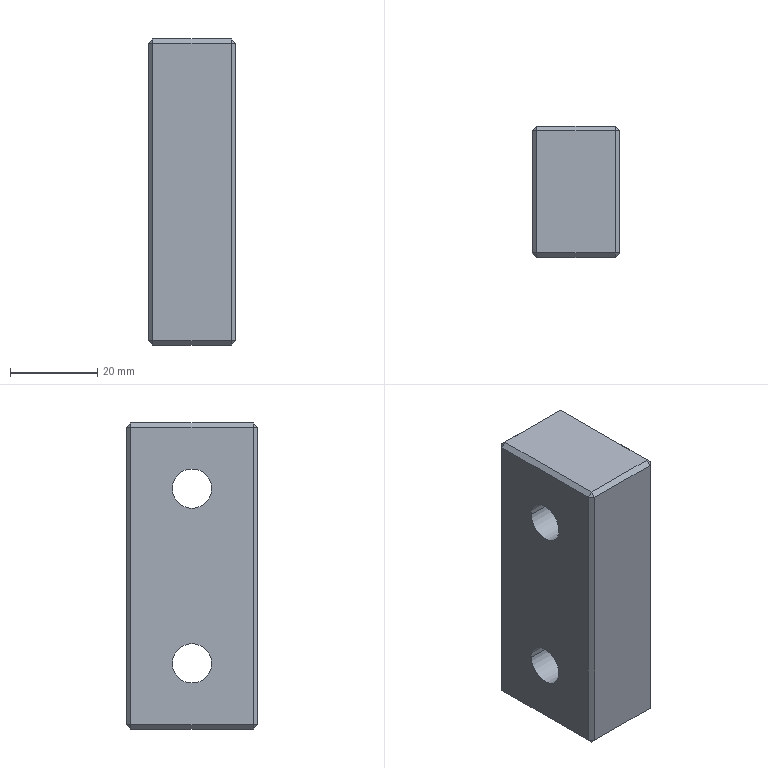Part | Creo | 1 solid | 36 faces | box 20 x 30 x 70 mm | volume 37595 mm3 | plane 28 | cylinder 8 | commonest cylinder face diameters 9 x4 14 x4
STEP:
#1=CARTESIAN_POINT('',(325.,-319.,-34.));
#2=VERTEX_POINT('',#1);
#3=CARTESIAN_POINT('',(325.,-291.,-34.));
#4=VERTEX_POINT('',#3);
#5=CARTESIAN_POINT('',(325.,-319.,-34.));
#6=DIRECTION('',(0.,1.,0.));
#7=VECTOR('',#6,28.);
#8=LINE('',#5,#7);
#9=EDGE_CURVE('',#2,#4,#8,.T.);
#10=ORIENTED_EDGE('',*,*,#9,.T.);
#11=CARTESIAN_POINT('',(325.,-291.,34.));
#12=VERTEX_POINT('',#11);
#13=CARTESIAN_POINT('',(325.,-291.,-34.));
#14=DIRECTION('',(0.,0.,1.));
#15=VECTOR('',#14,68.);
#16=LINE('',#13,#15);
#17=EDGE_CURVE('',#4,#12,#16,.T.);
#18=ORIENTED_EDGE('',*,*,#17,.T.);
#19=CARTESIAN_POINT('',(325.,-319.,34.));
#20=VERTEX_POINT('',#19);
#21=CARTESIAN_POINT('',(325.,-291.,34.));
#22=DIRECTION('',(0.,-1.,0.));
#23=VECTOR('',#22,28.);
#24=LINE('',#21,#23);
#25=EDGE_CURVE('',#12,#20,#24,.T.);
#26=ORIENTED_EDGE('',*,*,#25,.T.);
#27=CARTESIAN_POINT('',(325.,-319.,34.));
#28=DIRECTION('',(0.,0.,-1.));
#29=VECTOR('',#28,68.);
#30=LINE('',#27,#29);
#31=EDGE_CURVE('',#20,#2,#30,.T.);
#32=ORIENTED_EDGE('',*,*,#31,.T.);
#33=EDGE_LOOP('',(#10,#18,#26,#32));
#34=FACE_OUTER_BOUND('',#33,.F.);
#35=CARTESIAN_POINT('',(325.,-300.5,20.));
#36=VERTEX_POINT('',#35);
#37=CARTESIAN_POINT('',(325.,-309.5,20.));
#38=VERTEX_POINT('',#37);
#39=CARTESIAN_POINT('',(325.,-305.,20.));
#40=DIRECTION('',(1.,0.,0.));
#41=DIRECTION('',(0.,1.,0.));
#42=AXIS2_PLACEMENT_3D('',#39,#40,#41);
#43=CIRCLE('',#42,4.5);
#44=EDGE_CURVE('',#36,#38,#43,.T.);
#45=ORIENTED_EDGE('',*,*,#44,.F.);
#46=CARTESIAN_POINT('',(325.,-305.,20.));
#47=DIRECTION('',(1.,0.,0.));
#48=DIRECTION('',(0.,-1.,0.));
#49=AXIS2_PLACEMENT_3D('',#46,#47,#48);
#50=CIRCLE('',#49,4.5);
#51=EDGE_CURVE('',#38,#36,#50,.T.);
#52=ORIENTED_EDGE('',*,*,#51,.F.);
#53=EDGE_LOOP('',(#45,#52));
#54=FACE_BOUND('',#53,.F.);
#55=CARTESIAN_POINT('',(325.,-300.5,-20.));
#56=VERTEX_POINT('',#55);
#57=CARTESIAN_POINT('',(325.,-309.5,-20.));
#58=VERTEX_POINT('',#57);
#59=CARTESIAN_POINT('',(325.,-305.,-20.));
#60=DIRECTION('',(1.,0.,0.));
#61=DIRECTION('',(0.,1.,0.));
#62=AXIS2_PLACEMENT_3D('',#59,#60,#61);
#63=CIRCLE('',#62,4.5);
#64=EDGE_CURVE('',#56,#58,#63,.T.);
#65=ORIENTED_EDGE('',*,*,#64,.F.);
#66=CARTESIAN_POINT('',(325.,-305.,-20.));
#67=DIRECTION('',(1.,0.,0.));
#68=DIRECTION('',(0.,-1.,0.));
#69=AXIS2_PLACEMENT_3D('',#66,#67,#68);
#70=CIRCLE('',#69,4.5);
#71=EDGE_CURVE('',#58,#56,#70,.T.);
#72=ORIENTED_EDGE('',*,*,#71,.F.);
#73=EDGE_LOOP('',(#65,#72));
#74=FACE_BOUND('',#73,.F.);
#75=CARTESIAN_POINT('',(325.,20.,-120.5));
#76=DIRECTION('',(-1.,0.,0.));
#77=DIRECTION('',(0.,0.,-1.));
#78=AXIS2_PLACEMENT_3D('',#75,#76,#77);
#79=PLANE('',#78);
#80=ADVANCED_FACE('',(#34,#54,#74),#79,.T.);
#81=CARTESIAN_POINT('',(326.,-291.,-35.));
#82=VERTEX_POINT('',#81);
#83=CARTESIAN_POINT('',(326.,-291.,-35.));
#84=DIRECTION('',(-0.7071,0.,0.7071));
#85=VECTOR('',#84,1.414);
#86=LINE('',#83,#85);
#87=EDGE_CURVE('',#82,#4,#86,.T.);
#88=ORIENTED_EDGE('',*,*,#87,.T.);
#89=ORIENTED_EDGE('',*,*,#9,.F.);
#90=CARTESIAN_POINT('',(326.,-319.,-35.));
#91=VERTEX_POINT('',#90);
#92=CARTESIAN_POINT('',(326.,-319.,-35.));
#93=DIRECTION('',(-0.7071,0.,0.7071));
#94=VECTOR('',#93,1.414);
#95=LINE('',#92,#94);
#96=EDGE_CURVE('',#91,#2,#95,.T.);
#97=ORIENTED_EDGE('',*,*,#96,.F.);
#98=CARTESIAN_POINT('',(326.,-291.,-35.));
#99=DIRECTION('',(0.,-1.,0.));
#100=VECTOR('',#99,28.);
#101=LINE('',#98,#100);
#102=EDGE_CURVE('',#82,#91,#101,.T.);
#103=ORIENTED_EDGE('',*,*,#102,.F.);
#104=EDGE_LOOP('',(#88,#89,#97,#103));
#105=FACE_OUTER_BOUND('',#104,.F.);
#106=CARTESIAN_POINT('',(326.,20.,-35.));
#107=DIRECTION('',(-0.7071,0.,-0.7071));
#108=DIRECTION('',(0.7071,0.,-0.7071));
#109=AXIS2_PLACEMENT_3D('',#106,#107,#108);
#110=PLANE('',#109);
#111=ADVANCED_FACE('',(#105),#110,.T.);
#112=CARTESIAN_POINT('',(326.,-290.,-34.));
#113=VERTEX_POINT('',#112);
#114=CARTESIAN_POINT('',(325.,-291.,-34.));
#115=DIRECTION('',(0.7071,0.7071,0.));
#116=VECTOR('',#115,1.414);
#117=LINE('',#114,#116);
#118=EDGE_CURVE('',#4,#113,#117,.T.);
#119=ORIENTED_EDGE('',*,*,#118,.F.);
#120=ORIENTED_EDGE('',*,*,#87,.F.);
#121=CARTESIAN_POINT('',(326.,-290.,-34.));
#122=DIRECTION('',(0.,-0.7071,-0.7071));
#123=VECTOR('',#122,1.414);
#124=LINE('',#121,#123);
#125=EDGE_CURVE('',#113,#82,#124,.T.);
#126=ORIENTED_EDGE('',*,*,#125,.F.);
#127=EDGE_LOOP('',(#119,#120,#126));
#128=FACE_OUTER_BOUND('',#127,.F.);
#129=CARTESIAN_POINT('',(326.,-291.,-35.));
#130=DIRECTION('',(-0.5774,0.5774,-0.5774));
#131=DIRECTION('',(0.7071,0.,-0.7071));
#132=AXIS2_PLACEMENT_3D('',#129,#130,#131);
#133=PLANE('',#132);
#134=ADVANCED_FACE('',(#128),#133,.T.);
#135=ORIENTED_EDGE('',*,*,#118,.T.);
#136=CARTESIAN_POINT('',(326.,-290.,34.));
#137=VERTEX_POINT('',#136);
#138=CARTESIAN_POINT('',(326.,-290.,34.));
#139=DIRECTION('',(0.,0.,-1.));
#140=VECTOR('',#139,68.);
#141=LINE('',#138,#140);
#142=EDGE_CURVE('',#137,#113,#141,.T.);
#143=ORIENTED_EDGE('',*,*,#142,.F.);
#144=CARTESIAN_POINT('',(326.,-290.,34.));
#145=DIRECTION('',(-0.7071,-0.7071,0.));
#146=VECTOR('',#145,1.414);
#147=LINE('',#144,#146);
#148=EDGE_CURVE('',#137,#12,#147,.T.);
#149=ORIENTED_EDGE('',*,*,#148,.T.);
#150=ORIENTED_EDGE('',*,*,#17,.F.);
#151=EDGE_LOOP('',(#135,#143,#149,#150));
#152=FACE_OUTER_BOUND('',#151,.F.);
#153=CARTESIAN_POINT('',(326.,-290.,20.));
#154=DIRECTION('',(-0.7071,0.7071,0.));
#155=DIRECTION('',(-0.7071,-0.7071,0.));
#156=AXIS2_PLACEMENT_3D('',#153,#154,#155);
#157=PLANE('',#156);
#158=ADVANCED_FACE('',(#152),#157,.T.);
#159=CARTESIAN_POINT('',(344.,-290.,-34.));
#160=VERTEX_POINT('',#159);
#161=CARTESIAN_POINT('',(344.,-290.,34.));
#162=VERTEX_POINT('',#161);
#163=CARTESIAN_POINT('',(344.,-290.,-34.));
#164=DIRECTION('',(0.,0.,1.));
#165=VECTOR('',#164,68.);
#166=LINE('',#163,#165);
#167=EDGE_CURVE('',#160,#162,#166,.T.);
#168=ORIENTED_EDGE('',*,*,#167,.T.);
#169=CARTESIAN_POINT('',(344.,-290.,34.));
#170=DIRECTION('',(-1.,0.,0.));
#171=VECTOR('',#170,18.);
#172=LINE('',#169,#171);
#173=EDGE_CURVE('',#162,#137,#172,.T.);
#174=ORIENTED_EDGE('',*,*,#173,.T.);
#175=ORIENTED_EDGE('',*,*,#142,.T.);
#176=CARTESIAN_POINT('',(326.,-290.,-34.));
#177=DIRECTION('',(1.,0.,0.));
#178=VECTOR('',#177,18.);
#179=LINE('',#176,#178);
#180=EDGE_CURVE('',#113,#160,#179,.T.);
#181=ORIENTED_EDGE('',*,*,#180,.T.);
#182=EDGE_LOOP('',(#168,#174,#175,#181));
#183=FACE_OUTER_BOUND('',#182,.F.);
#184=CARTESIAN_POINT('',(335.,-290.,20.));
#185=DIRECTION('',(0.,-1.,0.));
#186=DIRECTION('',(0.,0.,1.));
#187=AXIS2_PLACEMENT_3D('',#184,#185,#186);
#188=PLANE('',#187);
#189=ADVANCED_FACE('',(#183),#188,.F.);
#190=CARTESIAN_POINT('',(345.,-291.,-34.));
#191=VERTEX_POINT('',#190);
#192=CARTESIAN_POINT('',(344.,-290.,-34.));
#193=DIRECTION('',(0.7071,-0.7071,0.));
#194=VECTOR('',#193,1.414);
#195=LINE('',#192,#194);
#196=EDGE_CURVE('',#160,#191,#195,.T.);
#197=ORIENTED_EDGE('',*,*,#196,.T.);
#198=CARTESIAN_POINT('',(345.,-291.,34.));
#199=VERTEX_POINT('',#198);
#200=CARTESIAN_POINT('',(345.,-291.,34.));
#201=DIRECTION('',(0.,0.,-1.));
#202=VECTOR('',#201,68.);
#203=LINE('',#200,#202);
#204=EDGE_CURVE('',#199,#191,#203,.T.);
#205=ORIENTED_EDGE('',*,*,#204,.F.);
#206=CARTESIAN_POINT('',(345.,-291.,34.));
#207=DIRECTION('',(-0.7071,0.7071,0.));
#208=VECTOR('',#207,1.414);
#209=LINE('',#206,#208);
#210=EDGE_CURVE('',#199,#162,#209,.T.);
#211=ORIENTED_EDGE('',*,*,#210,.T.);
#212=ORIENTED_EDGE('',*,*,#167,.F.);
#213=EDGE_LOOP('',(#197,#205,#211,#212));
#214=FACE_OUTER_BOUND('',#213,.F.);
#215=CARTESIAN_POINT('',(344.,-290.,20.));
#216=DIRECTION('',(0.7071,0.7071,0.));
#217=DIRECTION('',(-0.7071,0.7071,0.));
#218=AXIS2_PLACEMENT_3D('',#215,#216,#217);
#219=PLANE('',#218);
#220=ADVANCED_FACE('',(#214),#219,.T.);
#221=CARTESIAN_POINT('',(344.,-291.,-35.));
#222=VERTEX_POINT('',#221);
#223=CARTESIAN_POINT('',(345.,-291.,-34.));
#224=DIRECTION('',(-0.7071,0.,-0.7071));
#225=VECTOR('',#224,1.414);
#226=LINE('',#223,#225);
#227=EDGE_CURVE('',#191,#222,#226,.T.);
#228=ORIENTED_EDGE('',*,*,#227,.F.);
#229=ORIENTED_EDGE('',*,*,#196,.F.);
#230=CARTESIAN_POINT('',(344.,-291.,-35.));
#231=DIRECTION('',(0.,0.7071,0.7071));
#232=VECTOR('',#231,1.414);
#233=LINE('',#230,#232);
#234=EDGE_CURVE('',#222,#160,#233,.T.);
#235=ORIENTED_EDGE('',*,*,#234,.F.);
#236=EDGE_LOOP('',(#228,#229,#235));
#237=FACE_OUTER_BOUND('',#236,.F.);
#238=CARTESIAN_POINT('',(344.,-291.,-35.));
#239=DIRECTION('',(0.5774,0.5774,-0.5774));
#240=DIRECTION('',(0.7071,0.,0.7071));
#241=AXIS2_PLACEMENT_3D('',#238,#239,#240);
#242=PLANE('',#241);
#243=ADVANCED_FACE('',(#237),#242,.T.);
#244=ORIENTED_EDGE('',*,*,#227,.T.);
#245=CARTESIAN_POINT('',(344.,-319.,-35.));
#246=VERTEX_POINT('',#245);
#247=CARTESIAN_POINT('',(344.,-319.,-35.));
#248=DIRECTION('',(0.,1.,0.));
#249=VECTOR('',#248,28.);
#250=LINE('',#247,#249);
#251=EDGE_CURVE('',#246,#222,#250,.T.);
#252=ORIENTED_EDGE('',*,*,#251,.F.);
#253=CARTESIAN_POINT('',(345.,-319.,-34.));
#254=VERTEX_POINT('',#253);
#255=CARTESIAN_POINT('',(345.,-319.,-34.));
#256=DIRECTION('',(-0.7071,0.,-0.7071));
#257=VECTOR('',#256,1.414);
#258=LINE('',#255,#257);
#259=EDGE_CURVE('',#254,#246,#258,.T.);
#260=ORIENTED_EDGE('',*,*,#259,.F.);
#261=CARTESIAN_POINT('',(345.,-291.,-34.));
#262=DIRECTION('',(0.,-1.,0.));
#263=VECTOR('',#262,28.);
#264=LINE('',#261,#263);
#265=EDGE_CURVE('',#191,#254,#264,.T.);
#266=ORIENTED_EDGE('',*,*,#265,.F.);
#267=EDGE_LOOP('',(#244,#252,#260,#266));
#268=FACE_OUTER_BOUND('',#267,.F.);
#269=CARTESIAN_POINT('',(344.,20.,-35.));
#270=DIRECTION('',(0.7071,0.,-0.7071));
#271=DIRECTION('',(0.7071,0.,0.7071));
#272=AXIS2_PLACEMENT_3D('',#269,#270,#271);
#273=PLANE('',#272);
#274=ADVANCED_FACE('',(#268),#273,.T.);
#275=ORIENTED_EDGE('',*,*,#251,.T.);
#276=CARTESIAN_POINT('',(344.,-291.,-35.));
#277=DIRECTION('',(-1.,0.,0.));
#278=VECTOR('',#277,18.);
#279=LINE('',#276,#278);
#280=EDGE_CURVE('',#222,#82,#279,.T.);
#281=ORIENTED_EDGE('',*,*,#280,.T.);
#282=ORIENTED_EDGE('',*,*,#102,.T.);
#283=CARTESIAN_POINT('',(326.,-319.,-35.));
#284=DIRECTION('',(1.,0.,0.));
#285=VECTOR('',#284,18.);
#286=LINE('',#283,#285);
#287=EDGE_CURVE('',#91,#246,#286,.T.);
#288=ORIENTED_EDGE('',*,*,#287,.T.);
#289=EDGE_LOOP('',(#275,#281,#282,#288));
#290=FACE_OUTER_BOUND('',#289,.F.);
#291=CARTESIAN_POINT('',(0.,20.,-35.));
#292=DIRECTION('',(0.,0.,1.));
#293=DIRECTION('',(-1.,0.,0.));
#294=AXIS2_PLACEMENT_3D('',#291,#292,#293);
#295=PLANE('',#294);
#296=ADVANCED_FACE('',(#290),#295,.F.);
#297=ORIENTED_EDGE('',*,*,#234,.T.);
#298=ORIENTED_EDGE('',*,*,#180,.F.);
#299=ORIENTED_EDGE('',*,*,#125,.T.);
#300=ORIENTED_EDGE('',*,*,#280,.F.);
#301=EDGE_LOOP('',(#297,#298,#299,#300));
#302=FACE_OUTER_BOUND('',#301,.F.);
#303=CARTESIAN_POINT('',(335.,-290.,-34.));
#304=DIRECTION('',(0.,-0.7071,0.7071));
#305=DIRECTION('',(0.,0.7071,0.7071));
#306=AXIS2_PLACEMENT_3D('',#303,#304,#305);
#307=PLANE('',#306);
#308=ADVANCED_FACE('',(#302),#307,.F.);
#309=CARTESIAN_POINT('',(326.,-320.,-34.));
#310=VERTEX_POINT('',#309);
#311=CARTESIAN_POINT('',(326.,-319.,-35.));
#312=DIRECTION('',(0.,-0.7071,0.7071));
#313=VECTOR('',#312,1.414);
#314=LINE('',#311,#313);
#315=EDGE_CURVE('',#91,#310,#314,.T.);
#316=ORIENTED_EDGE('',*,*,#315,.T.);
#317=CARTESIAN_POINT('',(344.,-320.,-34.));
#318=VERTEX_POINT('',#317);
#319=CARTESIAN_POINT('',(344.,-320.,-34.));
#320=DIRECTION('',(-1.,0.,0.));
#321=VECTOR('',#320,18.);
#322=LINE('',#319,#321);
#323=EDGE_CURVE('',#318,#310,#322,.T.);
#324=ORIENTED_EDGE('',*,*,#323,.F.);
#325=CARTESIAN_POINT('',(344.,-320.,-34.));
#326=DIRECTION('',(0.,0.7071,-0.7071));
#327=VECTOR('',#326,1.414);
#328=LINE('',#325,#327);
#329=EDGE_CURVE('',#318,#246,#328,.T.);
#330=ORIENTED_EDGE('',*,*,#329,.T.);
#331=ORIENTED_EDGE('',*,*,#287,.F.);
#332=EDGE_LOOP('',(#316,#324,#330,#331));
#333=FACE_OUTER_BOUND('',#332,.F.);
#334=CARTESIAN_POINT('',(0.,-319.,-35.));
#335=DIRECTION('',(0.,-0.7071,-0.7071));
#336=DIRECTION('',(0.,-0.7071,0.7071));
#337=AXIS2_PLACEMENT_3D('',#334,#335,#336);
#338=PLANE('',#337);
#339=ADVANCED_FACE('',(#333),#338,.T.);
#340=ORIENTED_EDGE('',*,*,#96,.T.);
#341=CARTESIAN_POINT('',(326.,-320.,-34.));
#342=DIRECTION('',(-0.7071,0.7071,0.));
#343=VECTOR('',#342,1.414);
#344=LINE('',#341,#343);
#345=EDGE_CURVE('',#310,#2,#344,.T.);
#346=ORIENTED_EDGE('',*,*,#345,.F.);
#347=ORIENTED_EDGE('',*,*,#315,.F.);
#348=EDGE_LOOP('',(#340,#346,#347));
#349=FACE_OUTER_BOUND('',#348,.F.);
#350=CARTESIAN_POINT('',(326.,-320.,-34.));
#351=DIRECTION('',(-0.5774,-0.5774,-0.5774));
#352=DIRECTION('',(0.7071,0.,-0.7071));
#353=AXIS2_PLACEMENT_3D('',#350,#351,#352);
#354=PLANE('',#353);
#355=ADVANCED_FACE('',(#349),#354,.T.);
#356=ORIENTED_EDGE('',*,*,#345,.T.);
#357=ORIENTED_EDGE('',*,*,#31,.F.);
#358=CARTESIAN_POINT('',(326.,-320.,34.));
#359=VERTEX_POINT('',#358);
#360=CARTESIAN_POINT('',(325.,-319.,34.));
#361=DIRECTION('',(0.7071,-0.7071,0.));
#362=VECTOR('',#361,1.414);
#363=LINE('',#360,#362);
#364=EDGE_CURVE('',#20,#359,#363,.T.);
#365=ORIENTED_EDGE('',*,*,#364,.T.);
#366=CARTESIAN_POINT('',(326.,-320.,-34.));
#367=DIRECTION('',(0.,0.,1.));
#368=VECTOR('',#367,68.);
#369=LINE('',#366,#368);
#370=EDGE_CURVE('',#310,#359,#369,.T.);
#371=ORIENTED_EDGE('',*,*,#370,.F.);
#372=EDGE_LOOP('',(#356,#357,#365,#371));
#373=FACE_OUTER_BOUND('',#372,.F.);
#374=CARTESIAN_POINT('',(325.,-319.,-120.5));
#375=DIRECTION('',(0.7071,0.7071,0.));
#376=DIRECTION('',(-0.7071,0.7071,0.));
#377=AXIS2_PLACEMENT_3D('',#374,#375,#376);
#378=PLANE('',#377);
#379=ADVANCED_FACE('',(#373),#378,.F.);
#380=CARTESIAN_POINT('',(326.,-319.,35.));
#381=VERTEX_POINT('',#380);
#382=CARTESIAN_POINT('',(325.,-319.,34.));
#383=DIRECTION('',(0.7071,0.,0.7071));
#384=VECTOR('',#383,1.414);
#385=LINE('',#382,#384);
#386=EDGE_CURVE('',#20,#381,#385,.T.);
#387=ORIENTED_EDGE('',*,*,#386,.T.);
#388=CARTESIAN_POINT('',(326.,-320.,34.));
#389=DIRECTION('',(0.,0.7071,0.7071));
#390=VECTOR('',#389,1.414);
#391=LINE('',#388,#390);
#392=EDGE_CURVE('',#359,#381,#391,.T.);
#393=ORIENTED_EDGE('',*,*,#392,.F.);
#394=ORIENTED_EDGE('',*,*,#364,.F.);
#395=EDGE_LOOP('',(#387,#393,#394));
#396=FACE_OUTER_BOUND('',#395,.F.);
#397=CARTESIAN_POINT('',(326.,-320.,34.));
#398=DIRECTION('',(-0.5774,-0.5774,0.5774));
#399=DIRECTION('',(-0.7071,0.,-0.7071));
#400=AXIS2_PLACEMENT_3D('',#397,#398,#399);
#401=PLANE('',#400);
#402=ADVANCED_FACE('',(#396),#401,.T.);
#403=CARTESIAN_POINT('',(326.,-291.,35.));
#404=VERTEX_POINT('',#403);
#405=CARTESIAN_POINT('',(325.,-291.,34.));
#406=DIRECTION('',(0.7071,0.,0.7071));
#407=VECTOR('',#406,1.414);
#408=LINE('',#405,#407);
#409=EDGE_CURVE('',#12,#404,#408,.T.);
#410=ORIENTED_EDGE('',*,*,#409,.T.);
#411=CARTESIAN_POINT('',(326.,-319.,35.));
#412=DIRECTION('',(0.,1.,0.));
#413=VECTOR('',#412,28.);
#414=LINE('',#411,#413);
#415=EDGE_CURVE('',#381,#404,#414,.T.);
#416=ORIENTED_EDGE('',*,*,#415,.F.);
#417=ORIENTED_EDGE('',*,*,#386,.F.);
#418=ORIENTED_EDGE('',*,*,#25,.F.);
#419=EDGE_LOOP('',(#410,#416,#417,#418));
#420=FACE_OUTER_BOUND('',#419,.F.);
#421=CARTESIAN_POINT('',(325.,20.,34.));
#422=DIRECTION('',(0.7071,0.,-0.7071));
#423=DIRECTION('',(0.7071,0.,0.7071));
#424=AXIS2_PLACEMENT_3D('',#421,#422,#423);
#425=PLANE('',#424);
#426=ADVANCED_FACE('',(#420),#425,.F.);
#427=CARTESIAN_POINT('',(326.,-291.,35.));
#428=DIRECTION('',(0.,0.7071,-0.7071));
#429=VECTOR('',#428,1.414);
#430=LINE('',#427,#429);
#431=EDGE_CURVE('',#404,#137,#430,.T.);
#432=ORIENTED_EDGE('',*,*,#431,.F.);
#433=ORIENTED_EDGE('',*,*,#409,.F.);
#434=ORIENTED_EDGE('',*,*,#148,.F.);
#435=EDGE_LOOP('',(#432,#433,#434));
#436=FACE_OUTER_BOUND('',#435,.F.);
#437=CARTESIAN_POINT('',(326.,-290.,34.));
#438=DIRECTION('',(-0.5774,0.5774,0.5774));
#439=DIRECTION('',(-0.7071,0.,-0.7071));
#440=AXIS2_PLACEMENT_3D('',#437,#438,#439);
#441=PLANE('',#440);
#442=ADVANCED_FACE('',(#436),#441,.T.);
#443=CARTESIAN_POINT('',(344.,-291.,35.));
#444=VERTEX_POINT('',#443);
#445=CARTESIAN_POINT('',(344.,-290.,34.));
#446=DIRECTION('',(0.,-0.7071,0.7071));
#447=VECTOR('',#446,1.414);
#448=LINE('',#445,#447);
#449=EDGE_CURVE('',#162,#444,#448,.T.);
#450=ORIENTED_EDGE('',*,*,#449,.T.);
#451=CARTESIAN_POINT('',(326.,-291.,35.));
#452=DIRECTION('',(1.,0.,0.));
#453=VECTOR('',#452,18.);
#454=LINE('',#451,#453);
#455=EDGE_CURVE('',#404,#444,#454,.T.);
#456=ORIENTED_EDGE('',*,*,#455,.F.);
#457=ORIENTED_EDGE('',*,*,#431,.T.);
#458=ORIENTED_EDGE('',*,*,#173,.F.);
#459=EDGE_LOOP('',(#450,#456,#457,#458));
#460=FACE_OUTER_BOUND('',#459,.F.);
#461=CARTESIAN_POINT('',(0.,-291.,35.));
#462=DIRECTION('',(0.,0.7071,0.7071));
#463=DIRECTION('',(0.,0.7071,-0.7071));
#464=AXIS2_PLACEMENT_3D('',#461,#462,#463);
#465=PLANE('',#464);
#466=ADVANCED_FACE('',(#460),#465,.T.);
#467=ORIENTED_EDGE('',*,*,#210,.F.);
#468=CARTESIAN_POINT('',(344.,-291.,35.));
#469=DIRECTION('',(0.7071,0.,-0.7071));
#470=VECTOR('',#469,1.414);
#471=LINE('',#468,#470);
#472=EDGE_CURVE('',#444,#199,#471,.T.);
#473=ORIENTED_EDGE('',*,*,#472,.F.);
#474=ORIENTED_EDGE('',*,*,#449,.F.);
#475=EDGE_LOOP('',(#467,#473,#474));
#476=FACE_OUTER_BOUND('',#475,.F.);
#477=CARTESIAN_POINT('',(345.,-291.,34.));
#478=DIRECTION('',(0.5774,0.5774,0.5774));
#479=DIRECTION('',(-0.7071,0.,0.7071));
#480=AXIS2_PLACEMENT_3D('',#477,#478,#479);
#481=PLANE('',#480);
#482=ADVANCED_FACE('',(#476),#481,.T.);
#483=ORIENTED_EDGE('',*,*,#472,.T.);
#484=CARTESIAN_POINT('',(345.,-319.,34.));
#485=VERTEX_POINT('',#484);
#486=CARTESIAN_POINT('',(345.,-319.,34.));
#487=DIRECTION('',(0.,1.,0.));
#488=VECTOR('',#487,28.);
#489=LINE('',#486,#488);
#490=EDGE_CURVE('',#485,#199,#489,.T.);
#491=ORIENTED_EDGE('',*,*,#490,.F.);
#492=CARTESIAN_POINT('',(344.,-319.,35.));
#493=VERTEX_POINT('',#492);
#494=CARTESIAN_POINT('',(344.,-319.,35.));
#495=DIRECTION('',(0.7071,0.,-0.7071));
#496=VECTOR('',#495,1.414);
#497=LINE('',#494,#496);
#498=EDGE_CURVE('',#493,#485,#497,.T.);
#499=ORIENTED_EDGE('',*,*,#498,.F.);
#500=CARTESIAN_POINT('',(344.,-291.,35.));
#501=DIRECTION('',(0.,-1.,0.));
#502=VECTOR('',#501,28.);
#503=LINE('',#500,#502);
#504=EDGE_CURVE('',#444,#493,#503,.T.);
#505=ORIENTED_EDGE('',*,*,#504,.F.);
#506=EDGE_LOOP('',(#483,#491,#499,#505));
#507=FACE_OUTER_BOUND('',#506,.F.);
#508=CARTESIAN_POINT('',(345.,20.,34.));
#509=DIRECTION('',(-0.7071,0.,-0.7071));
#510=DIRECTION('',(0.7071,0.,-0.7071));
#511=AXIS2_PLACEMENT_3D('',#508,#509,#510);
#512=PLANE('',#511);
#513=ADVANCED_FACE('',(#507),#512,.F.);
#514=CARTESIAN_POINT('',(345.,-319.,-34.));
#515=DIRECTION('',(0.,0.,1.));
#516=VECTOR('',#515,68.);
#517=LINE('',#514,#516);
#518=EDGE_CURVE('',#254,#485,#517,.T.);
#519=ORIENTED_EDGE('',*,*,#518,.T.);
#520=ORIENTED_EDGE('',*,*,#490,.T.);
#521=ORIENTED_EDGE('',*,*,#204,.T.);
#522=ORIENTED_EDGE('',*,*,#265,.T.);
#523=EDGE_LOOP('',(#519,#520,#521,#522));
#524=FACE_OUTER_BOUND('',#523,.F.);
#525=CARTESIAN_POINT('',(345.,-298.,-20.));
#526=VERTEX_POINT('',#525);
#527=CARTESIAN_POINT('',(345.,-312.,-20.));
#528=VERTEX_POINT('',#527);
#529=CARTESIAN_POINT('',(345.,-305.,-20.));
#530=DIRECTION('',(-1.,0.,0.));
#531=DIRECTION('',(0.,1.,0.));
#532=AXIS2_PLACEMENT_3D('',#529,#530,#531);
#533=CIRCLE('',#532,7.);
#534=EDGE_CURVE('',#526,#528,#533,.T.);
#535=ORIENTED_EDGE('',*,*,#534,.F.);
#536=CARTESIAN_POINT('',(345.,-305.,-20.));
#537=DIRECTION('',(-1.,0.,0.));
#538=DIRECTION('',(0.,-1.,0.));
#539=AXIS2_PLACEMENT_3D('',#536,#537,#538);
#540=CIRCLE('',#539,7.);
#541=EDGE_CURVE('',#528,#526,#540,.T.);
#542=ORIENTED_EDGE('',*,*,#541,.F.);
#543=EDGE_LOOP('',(#535,#542));
#544=FACE_BOUND('',#543,.F.);
#545=CARTESIAN_POINT('',(345.,-298.,20.));
#546=VERTEX_POINT('',#545);
#547=CARTESIAN_POINT('',(345.,-312.,20.));
#548=VERTEX_POINT('',#547);
#549=CARTESIAN_POINT('',(345.,-305.,20.));
#550=DIRECTION('',(-1.,0.,0.));
#551=DIRECTION('',(0.,1.,0.));
#552=AXIS2_PLACEMENT_3D('',#549,#550,#551);
#553=CIRCLE('',#552,7.);
#554=EDGE_CURVE('',#546,#548,#553,.T.);
#555=ORIENTED_EDGE('',*,*,#554,.F.);
#556=CARTESIAN_POINT('',(345.,-305.,20.));
#557=DIRECTION('',(-1.,0.,0.));
#558=DIRECTION('',(0.,-1.,0.));
#559=AXIS2_PLACEMENT_3D('',#556,#557,#558);
#560=CIRCLE('',#559,7.);
#561=EDGE_CURVE('',#548,#546,#560,.T.);
#562=ORIENTED_EDGE('',*,*,#561,.F.);
#563=EDGE_LOOP('',(#555,#562));
#564=FACE_BOUND('',#563,.F.);
#565=CARTESIAN_POINT('',(345.,20.,-120.5));
#566=DIRECTION('',(1.,0.,0.));
#567=DIRECTION('',(0.,0.,1.));
#568=AXIS2_PLACEMENT_3D('',#565,#566,#567);
#569=PLANE('',#568);
#570=ADVANCED_FACE('',(#524,#544,#564),#569,.T.);
#571=CARTESIAN_POINT('',(345.,-319.,-34.));
#572=DIRECTION('',(-0.7071,-0.7071,0.));
#573=VECTOR('',#572,1.414);
#574=LINE('',#571,#573);
#575=EDGE_CURVE('',#254,#318,#574,.T.);
#576=ORIENTED_EDGE('',*,*,#575,.T.);
#577=CARTESIAN_POINT('',(344.,-320.,34.));
#578=VERTEX_POINT('',#577);
#579=CARTESIAN_POINT('',(344.,-320.,34.));
#580=DIRECTION('',(0.,0.,-1.));
#581=VECTOR('',#580,68.);
#582=LINE('',#579,#581);
#583=EDGE_CURVE('',#578,#318,#582,.T.);
#584=ORIENTED_EDGE('',*,*,#583,.F.);
#585=CARTESIAN_POINT('',(344.,-320.,34.));
#586=DIRECTION('',(0.7071,0.7071,0.));
#587=VECTOR('',#586,1.414);
#588=LINE('',#585,#587);
#589=EDGE_CURVE('',#578,#485,#588,.T.);
#590=ORIENTED_EDGE('',*,*,#589,.T.);
#591=ORIENTED_EDGE('',*,*,#518,.F.);
#592=EDGE_LOOP('',(#576,#584,#590,#591));
#593=FACE_OUTER_BOUND('',#592,.F.);
#594=CARTESIAN_POINT('',(345.,-319.,-120.5));
#595=DIRECTION('',(-0.7071,0.7071,0.));
#596=DIRECTION('',(-0.7071,-0.7071,0.));
#597=AXIS2_PLACEMENT_3D('',#594,#595,#596);
#598=PLANE('',#597);
#599=ADVANCED_FACE('',(#593),#598,.F.);
#600=ORIENTED_EDGE('',*,*,#329,.F.);
#601=ORIENTED_EDGE('',*,*,#575,.F.);
#602=ORIENTED_EDGE('',*,*,#259,.T.);
#603=EDGE_LOOP('',(#600,#601,#602));
#604=FACE_OUTER_BOUND('',#603,.F.);
#605=CARTESIAN_POINT('',(344.,-320.,-34.));
#606=DIRECTION('',(0.5774,-0.5774,-0.5774));
#607=DIRECTION('',(0.7071,0.,0.7071));
#608=AXIS2_PLACEMENT_3D('',#605,#606,#607);
#609=PLANE('',#608);
#610=ADVANCED_FACE('',(#604),#609,.T.);
#611=ORIENTED_EDGE('',*,*,#583,.T.);
#612=ORIENTED_EDGE('',*,*,#323,.T.);
#613=ORIENTED_EDGE('',*,*,#370,.T.);
#614=CARTESIAN_POINT('',(326.,-320.,34.));
#615=DIRECTION('',(1.,0.,0.));
#616=VECTOR('',#615,18.);
#617=LINE('',#614,#616);
#618=EDGE_CURVE('',#359,#578,#617,.T.);
#619=ORIENTED_EDGE('',*,*,#618,.T.);
#620=EDGE_LOOP('',(#611,#612,#613,#619));
#621=FACE_OUTER_BOUND('',#620,.F.);
#622=CARTESIAN_POINT('',(335.,-320.,20.));
#623=DIRECTION('',(0.,-1.,0.));
#624=DIRECTION('',(0.,0.,1.));
#625=AXIS2_PLACEMENT_3D('',#622,#623,#624);
#626=PLANE('',#625);
#627=ADVANCED_FACE('',(#621),#626,.T.);
#628=CARTESIAN_POINT('',(344.,-319.,35.));
#629=DIRECTION('',(0.,-0.7071,-0.7071));
#630=VECTOR('',#629,1.414);
#631=LINE('',#628,#630);
#632=EDGE_CURVE('',#493,#578,#631,.T.);
#633=ORIENTED_EDGE('',*,*,#632,.T.);
#634=ORIENTED_EDGE('',*,*,#618,.F.);
#635=ORIENTED_EDGE('',*,*,#392,.T.);
#636=CARTESIAN_POINT('',(344.,-319.,35.));
#637=DIRECTION('',(-1.,0.,0.));
#638=VECTOR('',#637,18.);
#639=LINE('',#636,#638);
#640=EDGE_CURVE('',#493,#381,#639,.T.);
#641=ORIENTED_EDGE('',*,*,#640,.F.);
#642=EDGE_LOOP('',(#633,#634,#635,#641));
#643=FACE_OUTER_BOUND('',#642,.F.);
#644=CARTESIAN_POINT('',(335.,-320.,34.));
#645=DIRECTION('',(0.,0.7071,-0.7071));
#646=DIRECTION('',(0.,-0.7071,-0.7071));
#647=AXIS2_PLACEMENT_3D('',#644,#645,#646);
#648=PLANE('',#647);
#649=ADVANCED_FACE('',(#643),#648,.F.);
#650=ORIENTED_EDGE('',*,*,#589,.F.);
#651=ORIENTED_EDGE('',*,*,#632,.F.);
#652=ORIENTED_EDGE('',*,*,#498,.T.);
#653=EDGE_LOOP('',(#650,#651,#652));
#654=FACE_OUTER_BOUND('',#653,.F.);
#655=CARTESIAN_POINT('',(344.,-319.,35.));
#656=DIRECTION('',(0.5774,-0.5774,0.5774));
#657=DIRECTION('',(-0.7071,0.,0.7071));
#658=AXIS2_PLACEMENT_3D('',#655,#656,#657);
#659=PLANE('',#658);
#660=ADVANCED_FACE('',(#654),#659,.T.);
#661=ORIENTED_EDGE('',*,*,#415,.T.);
#662=ORIENTED_EDGE('',*,*,#455,.T.);
#663=ORIENTED_EDGE('',*,*,#504,.T.);
#664=ORIENTED_EDGE('',*,*,#640,.T.);
#665=EDGE_LOOP('',(#661,#662,#663,#664));
#666=FACE_OUTER_BOUND('',#665,.F.);
#667=CARTESIAN_POINT('',(0.,20.,35.));
#668=DIRECTION('',(0.,0.,1.));
#669=DIRECTION('',(-1.,0.,0.));
#670=AXIS2_PLACEMENT_3D('',#667,#668,#669);
#671=PLANE('',#670);
#672=ADVANCED_FACE('',(#666),#671,.T.);
#673=ORIENTED_EDGE('',*,*,#534,.T.);
#674=CARTESIAN_POINT('',(336.,-312.,-20.));
#675=VERTEX_POINT('',#674);
#676=CARTESIAN_POINT('',(336.,-312.,-20.));
#677=DIRECTION('',(1.,0.,0.));
#678=VECTOR('',#677,9.);
#679=LINE('',#676,#678);
#680=EDGE_CURVE('',#675,#528,#679,.T.);
#681=ORIENTED_EDGE('',*,*,#680,.F.);
#682=CARTESIAN_POINT('',(336.,-298.,-20.));
#683=VERTEX_POINT('',#682);
#684=CARTESIAN_POINT('',(336.,-305.,-20.));
#685=DIRECTION('',(1.,0.,0.));
#686=DIRECTION('',(0.,-1.,0.));
#687=AXIS2_PLACEMENT_3D('',#684,#685,#686);
#688=CIRCLE('',#687,7.);
#689=EDGE_CURVE('',#675,#683,#688,.T.);
#690=ORIENTED_EDGE('',*,*,#689,.T.);
#691=CARTESIAN_POINT('',(336.,-298.,-20.));
#692=DIRECTION('',(1.,0.,0.));
#693=VECTOR('',#692,9.);
#694=LINE('',#691,#693);
#695=EDGE_CURVE('',#683,#526,#694,.T.);
#696=ORIENTED_EDGE('',*,*,#695,.T.);
#697=EDGE_LOOP('',(#673,#681,#690,#696));
#698=FACE_OUTER_BOUND('',#697,.F.);
#699=CARTESIAN_POINT('',(336.,-305.,-20.));
#700=DIRECTION('',(1.,0.,0.));
#701=DIRECTION('',(0.,1.,0.));
#702=AXIS2_PLACEMENT_3D('',#699,#700,#701);
#703=CYLINDRICAL_SURFACE('',#702,7.);
#704=ADVANCED_FACE('',(#698),#703,.F.);
#705=ORIENTED_EDGE('',*,*,#541,.T.);
#706=ORIENTED_EDGE('',*,*,#695,.F.);
#707=CARTESIAN_POINT('',(336.,-305.,-20.));
#708=DIRECTION('',(1.,0.,0.));
#709=DIRECTION('',(0.,1.,0.));
#710=AXIS2_PLACEMENT_3D('',#707,#708,#709);
#711=CIRCLE('',#710,7.);
#712=EDGE_CURVE('',#683,#675,#711,.T.);
#713=ORIENTED_EDGE('',*,*,#712,.T.);
#714=ORIENTED_EDGE('',*,*,#680,.T.);
#715=EDGE_LOOP('',(#705,#706,#713,#714));
#716=FACE_OUTER_BOUND('',#715,.F.);
#717=CARTESIAN_POINT('',(336.,-305.,-20.));
#718=DIRECTION('',(1.,0.,0.));
#719=DIRECTION('',(0.,1.,0.));
#720=AXIS2_PLACEMENT_3D('',#717,#718,#719);
#721=CYLINDRICAL_SURFACE('',#720,7.);
#722=ADVANCED_FACE('',(#716),#721,.F.);
#723=ORIENTED_EDGE('',*,*,#712,.F.);
#724=ORIENTED_EDGE('',*,*,#689,.F.);
#725=EDGE_LOOP('',(#723,#724));
#726=FACE_OUTER_BOUND('',#725,.F.);
#727=CARTESIAN_POINT('',(336.,-300.5,-20.));
#728=VERTEX_POINT('',#727);
#729=CARTESIAN_POINT('',(336.,-309.5,-20.));
#730=VERTEX_POINT('',#729);
#731=CARTESIAN_POINT('',(336.,-305.,-20.));
#732=DIRECTION('',(-1.,0.,0.));
#733=DIRECTION('',(0.,1.,0.));
#734=AXIS2_PLACEMENT_3D('',#731,#732,#733);
#735=CIRCLE('',#734,4.5);
#736=EDGE_CURVE('',#728,#730,#735,.T.);
#737=ORIENTED_EDGE('',*,*,#736,.F.);
#738=CARTESIAN_POINT('',(336.,-305.,-20.));
#739=DIRECTION('',(-1.,0.,0.));
#740=DIRECTION('',(0.,-1.,0.));
#741=AXIS2_PLACEMENT_3D('',#738,#739,#740);
#742=CIRCLE('',#741,4.5);
#743=EDGE_CURVE('',#730,#728,#742,.T.);
#744=ORIENTED_EDGE('',*,*,#743,.F.);
#745=EDGE_LOOP('',(#737,#744));
#746=FACE_BOUND('',#745,.F.);
#747=CARTESIAN_POINT('',(336.,-305.,-20.));
#748=DIRECTION('',(-1.,0.,0.));
#749=DIRECTION('',(0.,-1.,0.));
#750=AXIS2_PLACEMENT_3D('',#747,#748,#749);
#751=PLANE('',#750);
#752=ADVANCED_FACE('',(#726,#746),#751,.F.);
#753=ORIENTED_EDGE('',*,*,#736,.T.);
#754=CARTESIAN_POINT('',(325.,-309.5,-20.));
#755=DIRECTION('',(1.,0.,0.));
#756=VECTOR('',#755,11.);
#757=LINE('',#754,#756);
#758=EDGE_CURVE('',#58,#730,#757,.T.);
#759=ORIENTED_EDGE('',*,*,#758,.F.);
#760=ORIENTED_EDGE('',*,*,#71,.T.);
#761=CARTESIAN_POINT('',(325.,-300.5,-20.));
#762=DIRECTION('',(1.,0.,0.));
#763=VECTOR('',#762,11.);
#764=LINE('',#761,#763);
#765=EDGE_CURVE('',#56,#728,#764,.T.);
#766=ORIENTED_EDGE('',*,*,#765,.T.);
#767=EDGE_LOOP('',(#753,#759,#760,#766));
#768=FACE_OUTER_BOUND('',#767,.F.);
#769=CARTESIAN_POINT('',(325.,-305.,-20.));
#770=DIRECTION('',(1.,0.,0.));
#771=DIRECTION('',(0.,1.,0.));
#772=AXIS2_PLACEMENT_3D('',#769,#770,#771);
#773=CYLINDRICAL_SURFACE('',#772,4.5);
#774=ADVANCED_FACE('',(#768),#773,.F.);
#775=ORIENTED_EDGE('',*,*,#743,.T.);
#776=ORIENTED_EDGE('',*,*,#765,.F.);
#777=ORIENTED_EDGE('',*,*,#64,.T.);
#778=ORIENTED_EDGE('',*,*,#758,.T.);
#779=EDGE_LOOP('',(#775,#776,#777,#778));
#780=FACE_OUTER_BOUND('',#779,.F.);
#781=CARTESIAN_POINT('',(325.,-305.,-20.));
#782=DIRECTION('',(1.,0.,0.));
#783=DIRECTION('',(0.,1.,0.));
#784=AXIS2_PLACEMENT_3D('',#781,#782,#783);
#785=CYLINDRICAL_SURFACE('',#784,4.5);
#786=ADVANCED_FACE('',(#780),#785,.F.);
#787=ORIENTED_EDGE('',*,*,#554,.T.);
#788=CARTESIAN_POINT('',(336.,-312.,20.));
#789=VERTEX_POINT('',#788);
#790=CARTESIAN_POINT('',(336.,-312.,20.));
#791=DIRECTION('',(1.,0.,0.));
#792=VECTOR('',#791,9.);
#793=LINE('',#790,#792);
#794=EDGE_CURVE('',#789,#548,#793,.T.);
#795=ORIENTED_EDGE('',*,*,#794,.F.);
#796=CARTESIAN_POINT('',(336.,-298.,20.));
#797=VERTEX_POINT('',#796);
#798=CARTESIAN_POINT('',(336.,-305.,20.));
#799=DIRECTION('',(1.,0.,0.));
#800=DIRECTION('',(0.,-1.,0.));
#801=AXIS2_PLACEMENT_3D('',#798,#799,#800);
#802=CIRCLE('',#801,7.);
#803=EDGE_CURVE('',#789,#797,#802,.T.);
#804=ORIENTED_EDGE('',*,*,#803,.T.);
#805=CARTESIAN_POINT('',(336.,-298.,20.));
#806=DIRECTION('',(1.,0.,0.));
#807=VECTOR('',#806,9.);
#808=LINE('',#805,#807);
#809=EDGE_CURVE('',#797,#546,#808,.T.);
#810=ORIENTED_EDGE('',*,*,#809,.T.);
#811=EDGE_LOOP('',(#787,#795,#804,#810));
#812=FACE_OUTER_BOUND('',#811,.F.);
#813=CARTESIAN_POINT('',(336.,-305.,20.));
#814=DIRECTION('',(1.,0.,0.));
#815=DIRECTION('',(0.,1.,0.));
#816=AXIS2_PLACEMENT_3D('',#813,#814,#815);
#817=CYLINDRICAL_SURFACE('',#816,7.);
#818=ADVANCED_FACE('',(#812),#817,.F.);
#819=ORIENTED_EDGE('',*,*,#561,.T.);
#820=ORIENTED_EDGE('',*,*,#809,.F.);
#821=CARTESIAN_POINT('',(336.,-305.,20.));
#822=DIRECTION('',(1.,0.,0.));
#823=DIRECTION('',(0.,1.,0.));
#824=AXIS2_PLACEMENT_3D('',#821,#822,#823);
#825=CIRCLE('',#824,7.);
#826=EDGE_CURVE('',#797,#789,#825,.T.);
#827=ORIENTED_EDGE('',*,*,#826,.T.);
#828=ORIENTED_EDGE('',*,*,#794,.T.);
#829=EDGE_LOOP('',(#819,#820,#827,#828));
#830=FACE_OUTER_BOUND('',#829,.F.);
#831=CARTESIAN_POINT('',(336.,-305.,20.));
#832=DIRECTION('',(1.,0.,0.));
#833=DIRECTION('',(0.,1.,0.));
#834=AXIS2_PLACEMENT_3D('',#831,#832,#833);
#835=CYLINDRICAL_SURFACE('',#834,7.);
#836=ADVANCED_FACE('',(#830),#835,.F.);
#837=ORIENTED_EDGE('',*,*,#826,.F.);
#838=ORIENTED_EDGE('',*,*,#803,.F.);
#839=EDGE_LOOP('',(#837,#838));
#840=FACE_OUTER_BOUND('',#839,.F.);
#841=CARTESIAN_POINT('',(336.,-300.5,20.));
#842=VERTEX_POINT('',#841);
#843=CARTESIAN_POINT('',(336.,-309.5,20.));
#844=VERTEX_POINT('',#843);
#845=CARTESIAN_POINT('',(336.,-305.,20.));
#846=DIRECTION('',(-1.,0.,0.));
#847=DIRECTION('',(0.,1.,0.));
#848=AXIS2_PLACEMENT_3D('',#845,#846,#847);
#849=CIRCLE('',#848,4.5);
#850=EDGE_CURVE('',#842,#844,#849,.T.);
#851=ORIENTED_EDGE('',*,*,#850,.F.);
#852=CARTESIAN_POINT('',(336.,-305.,20.));
#853=DIRECTION('',(-1.,0.,0.));
#854=DIRECTION('',(0.,-1.,0.));
#855=AXIS2_PLACEMENT_3D('',#852,#853,#854);
#856=CIRCLE('',#855,4.5);
#857=EDGE_CURVE('',#844,#842,#856,.T.);
#858=ORIENTED_EDGE('',*,*,#857,.F.);
#859=EDGE_LOOP('',(#851,#858));
#860=FACE_BOUND('',#859,.F.);
#861=CARTESIAN_POINT('',(336.,-305.,20.));
#862=DIRECTION('',(-1.,0.,0.));
#863=DIRECTION('',(0.,-1.,0.));
#864=AXIS2_PLACEMENT_3D('',#861,#862,#863);
#865=PLANE('',#864);
#866=ADVANCED_FACE('',(#840,#860),#865,.F.);
#867=ORIENTED_EDGE('',*,*,#850,.T.);
#868=CARTESIAN_POINT('',(325.,-309.5,20.));
#869=DIRECTION('',(1.,0.,0.));
#870=VECTOR('',#869,11.);
#871=LINE('',#868,#870);
#872=EDGE_CURVE('',#38,#844,#871,.T.);
#873=ORIENTED_EDGE('',*,*,#872,.F.);
#874=ORIENTED_EDGE('',*,*,#51,.T.);
#875=CARTESIAN_POINT('',(325.,-300.5,20.));
#876=DIRECTION('',(1.,0.,0.));
#877=VECTOR('',#876,11.);
#878=LINE('',#875,#877);
#879=EDGE_CURVE('',#36,#842,#878,.T.);
#880=ORIENTED_EDGE('',*,*,#879,.T.);
#881=EDGE_LOOP('',(#867,#873,#874,#880));
#882=FACE_OUTER_BOUND('',#881,.F.);
#883=CARTESIAN_POINT('',(325.,-305.,20.));
#884=DIRECTION('',(1.,0.,0.));
#885=DIRECTION('',(0.,1.,0.));
#886=AXIS2_PLACEMENT_3D('',#883,#884,#885);
#887=CYLINDRICAL_SURFACE('',#886,4.5);
#888=ADVANCED_FACE('',(#882),#887,.F.);
#889=ORIENTED_EDGE('',*,*,#857,.T.);
#890=ORIENTED_EDGE('',*,*,#879,.F.);
#891=ORIENTED_EDGE('',*,*,#44,.T.);
#892=ORIENTED_EDGE('',*,*,#872,.T.);
#893=EDGE_LOOP('',(#889,#890,#891,#892));
#894=FACE_OUTER_BOUND('',#893,.F.);
#895=CARTESIAN_POINT('',(325.,-305.,20.));
#896=DIRECTION('',(1.,0.,0.));
#897=DIRECTION('',(0.,1.,0.));
#898=AXIS2_PLACEMENT_3D('',#895,#896,#897);
#899=CYLINDRICAL_SURFACE('',#898,4.5);
#900=ADVANCED_FACE('',(#894),#899,.F.);
#901=CLOSED_SHELL('',(#80,#111,#134,#158,#189,#220,#243,#274,#296,#308,#339,#355,#379,#402,#426,#442,#466,#482,#513,#570,#599,#610,#627,#649,#660,#672,#704,#722,#752,#774,#786,#818,#836,#866,#888,#900));
#902=MANIFOLD_SOLID_BREP('',#901);
#903=(LENGTH_UNIT()NAMED_UNIT(*)SI_UNIT(.MILLI.,.METRE.));
#904=UNCERTAINTY_MEASURE_WITH_UNIT(LENGTH_MEASURE(0.007874),#903,'','');
#905=(NAMED_UNIT(*)PLANE_ANGLE_UNIT()SI_UNIT($,.RADIAN.));
#906=PLANE_ANGLE_MEASURE_WITH_UNIT(PLANE_ANGLE_MEASURE(0.01745),#905);
#907=(CONVERSION_BASED_UNIT('DEGREE',#906)NAMED_UNIT(*)PLANE_ANGLE_UNIT());
#908=(NAMED_UNIT(*)SI_UNIT($,.STERADIAN.)SOLID_ANGLE_UNIT());
#909=(GEOMETRIC_REPRESENTATION_CONTEXT(3)GLOBAL_UNCERTAINTY_ASSIGNED_CONTEXT((#904))GLOBAL_UNIT_ASSIGNED_CONTEXT((#903,#907,#908))REPRESENTATION_CONTEXT('',''));
#910=ADVANCED_BREP_SHAPE_REPRESENTATION('',(#902),#909);